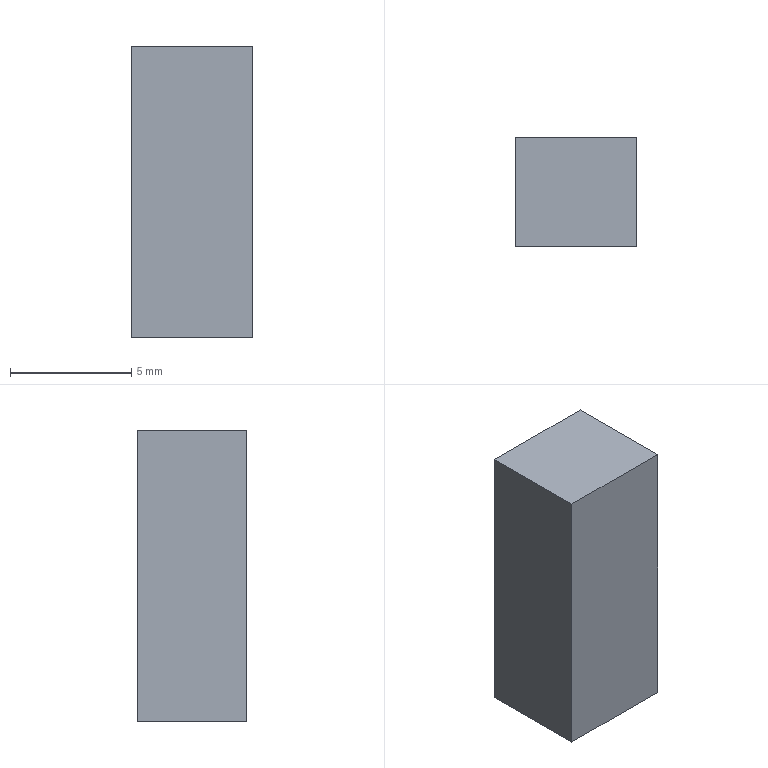Part | STEP file | Cuon T phu H01_7 | 1 solid | 6 faces | box 5 x 4.5 x 12 mm | volume 270 mm3 | plane 6
STEP:
#1=CARTESIAN_POINT('',(0.,0.,0.));
#2=DIRECTION('',(0.,0.,1.));
#3=DIRECTION('',(1.,0.,0.));
#4=AXIS2_PLACEMENT_3D('',#1,#2,#3);
#5=CARTESIAN_POINT('',(-2.5,2.25,-6.));
#6=VERTEX_POINT('',#5);
#7=CARTESIAN_POINT('',(-2.5,-2.25,-6.));
#8=VERTEX_POINT('',#7);
#9=CARTESIAN_POINT('',(-2.5,2.25,-6.));
#10=DIRECTION('',(0.,-1.,0.));
#11=VECTOR('',#10,1.);
#12=LINE('',#9,#11);
#13=CARTESIAN_POINT('',(-2.5,2.25,6.));
#14=DIRECTION('',(1.,0.,0.));
#15=DIRECTION('',(0.,1.,0.));
#16=AXIS2_PLACEMENT_3D('',#13,#14,#15);
#17=PLANE('',#16);
#18=CARTESIAN_POINT('',(0.,-12.));
#19=DIRECTION('',(-1.,0.));
#20=VECTOR('',#19,1.);
#21=LINE('',#18,#20);
#22=(GEOMETRIC_REPRESENTATION_CONTEXT(2)PARAMETRIC_REPRESENTATION_CONTEXT()REPRESENTATION_CONTEXT('',''));
#23=DEFINITIONAL_REPRESENTATION('',(#21),#22);
#24=PCURVE('',#17,#23);
#25=CARTESIAN_POINT('',(0.,0.,-6.));
#26=DIRECTION('',(0.,0.,1.));
#27=DIRECTION('',(1.,0.,0.));
#28=AXIS2_PLACEMENT_3D('',#25,#26,#27);
#29=PLANE('',#28);
#30=CARTESIAN_POINT('',(-2.5,2.25));
#31=DIRECTION('',(0.,-1.));
#32=VECTOR('',#31,1.);
#33=LINE('',#30,#32);
#34=(GEOMETRIC_REPRESENTATION_CONTEXT(2)PARAMETRIC_REPRESENTATION_CONTEXT()REPRESENTATION_CONTEXT('',''));
#35=DEFINITIONAL_REPRESENTATION('',(#33),#34);
#36=PCURVE('',#29,#35);
#37=SURFACE_CURVE('',#12,(#24,#36),.PCURVE_S1.);
#38=EDGE_CURVE('',#6,#8,#37,.T.);
#39=ORIENTED_EDGE('',*,*,#38,.T.);
#40=CARTESIAN_POINT('',(-2.5,-2.25,6.));
#41=VERTEX_POINT('',#40);
#42=CARTESIAN_POINT('',(-2.5,-2.25,6.));
#43=DIRECTION('',(0.,0.,-1.));
#44=VECTOR('',#43,1.);
#45=LINE('',#42,#44);
#46=CARTESIAN_POINT('',(-4.5,0.));
#47=DIRECTION('',(0.,-1.));
#48=VECTOR('',#47,1.);
#49=LINE('',#46,#48);
#50=(GEOMETRIC_REPRESENTATION_CONTEXT(2)PARAMETRIC_REPRESENTATION_CONTEXT()REPRESENTATION_CONTEXT('',''));
#51=DEFINITIONAL_REPRESENTATION('',(#49),#50);
#52=PCURVE('',#17,#51);
#53=CARTESIAN_POINT('',(-2.5,-2.25,6.));
#54=DIRECTION('',(0.,1.,0.));
#55=DIRECTION('',(0.,0.,1.));
#56=AXIS2_PLACEMENT_3D('',#53,#54,#55);
#57=PLANE('',#56);
#58=CARTESIAN_POINT('',(0.,0.));
#59=DIRECTION('',(-1.,0.));
#60=VECTOR('',#59,1.);
#61=LINE('',#58,#60);
#62=(GEOMETRIC_REPRESENTATION_CONTEXT(2)PARAMETRIC_REPRESENTATION_CONTEXT()REPRESENTATION_CONTEXT('',''));
#63=DEFINITIONAL_REPRESENTATION('',(#61),#62);
#64=PCURVE('',#57,#63);
#65=SURFACE_CURVE('',#45,(#52,#64),.PCURVE_S1.);
#66=EDGE_CURVE('',#41,#8,#65,.T.);
#67=ORIENTED_EDGE('',*,*,#66,.F.);
#68=CARTESIAN_POINT('',(-2.5,2.25,6.));
#69=VERTEX_POINT('',#68);
#70=CARTESIAN_POINT('',(-2.5,2.25,6.));
#71=DIRECTION('',(0.,-1.,0.));
#72=VECTOR('',#71,1.);
#73=LINE('',#70,#72);
#74=CARTESIAN_POINT('',(0.,0.));
#75=DIRECTION('',(-1.,0.));
#76=VECTOR('',#75,1.);
#77=LINE('',#74,#76);
#78=(GEOMETRIC_REPRESENTATION_CONTEXT(2)PARAMETRIC_REPRESENTATION_CONTEXT()REPRESENTATION_CONTEXT('',''));
#79=DEFINITIONAL_REPRESENTATION('',(#77),#78);
#80=PCURVE('',#17,#79);
#81=CARTESIAN_POINT('',(0.,0.,6.));
#82=DIRECTION('',(0.,0.,1.));
#83=DIRECTION('',(1.,0.,0.));
#84=AXIS2_PLACEMENT_3D('',#81,#82,#83);
#85=PLANE('',#84);
#86=CARTESIAN_POINT('',(-2.5,2.25));
#87=DIRECTION('',(0.,-1.));
#88=VECTOR('',#87,1.);
#89=LINE('',#86,#88);
#90=(GEOMETRIC_REPRESENTATION_CONTEXT(2)PARAMETRIC_REPRESENTATION_CONTEXT()REPRESENTATION_CONTEXT('',''));
#91=DEFINITIONAL_REPRESENTATION('',(#89),#90);
#92=PCURVE('',#85,#91);
#93=SURFACE_CURVE('',#73,(#80,#92),.PCURVE_S1.);
#94=EDGE_CURVE('',#69,#41,#93,.T.);
#95=ORIENTED_EDGE('',*,*,#94,.F.);
#96=CARTESIAN_POINT('',(-2.5,2.25,6.));
#97=DIRECTION('',(0.,0.,-1.));
#98=VECTOR('',#97,1.);
#99=LINE('',#96,#98);
#100=CARTESIAN_POINT('',(0.,0.));
#101=DIRECTION('',(0.,-1.));
#102=VECTOR('',#101,1.);
#103=LINE('',#100,#102);
#104=(GEOMETRIC_REPRESENTATION_CONTEXT(2)PARAMETRIC_REPRESENTATION_CONTEXT()REPRESENTATION_CONTEXT('',''));
#105=DEFINITIONAL_REPRESENTATION('',(#103),#104);
#106=PCURVE('',#17,#105);
#107=CARTESIAN_POINT('',(-2.5,2.25,6.));
#108=DIRECTION('',(0.,-1.,0.));
#109=DIRECTION('',(0.,0.,-1.));
#110=AXIS2_PLACEMENT_3D('',#107,#108,#109);
#111=PLANE('',#110);
#112=CARTESIAN_POINT('',(0.,0.));
#113=DIRECTION('',(1.,0.));
#114=VECTOR('',#113,1.);
#115=LINE('',#112,#114);
#116=(GEOMETRIC_REPRESENTATION_CONTEXT(2)PARAMETRIC_REPRESENTATION_CONTEXT()REPRESENTATION_CONTEXT('',''));
#117=DEFINITIONAL_REPRESENTATION('',(#115),#116);
#118=PCURVE('',#111,#117);
#119=SURFACE_CURVE('',#99,(#106,#118),.PCURVE_S1.);
#120=EDGE_CURVE('',#69,#6,#119,.T.);
#121=ORIENTED_EDGE('',*,*,#120,.T.);
#122=EDGE_LOOP('',(#39,#67,#95,#121));
#123=FACE_BOUND('',#122,.T.);
#124=ADVANCED_FACE('',(#123),#17,.F.);
#125=CARTESIAN_POINT('',(2.5,-2.25,-6.));
#126=VERTEX_POINT('',#125);
#127=CARTESIAN_POINT('',(-2.5,-2.25,-6.));
#128=DIRECTION('',(1.,0.,0.));
#129=VECTOR('',#128,1.);
#130=LINE('',#127,#129);
#131=CARTESIAN_POINT('',(-12.,0.));
#132=DIRECTION('',(0.,1.));
#133=VECTOR('',#132,1.);
#134=LINE('',#131,#133);
#135=(GEOMETRIC_REPRESENTATION_CONTEXT(2)PARAMETRIC_REPRESENTATION_CONTEXT()REPRESENTATION_CONTEXT('',''));
#136=DEFINITIONAL_REPRESENTATION('',(#134),#135);
#137=PCURVE('',#57,#136);
#138=CARTESIAN_POINT('',(-2.5,-2.25));
#139=DIRECTION('',(1.,0.));
#140=VECTOR('',#139,1.);
#141=LINE('',#138,#140);
#142=(GEOMETRIC_REPRESENTATION_CONTEXT(2)PARAMETRIC_REPRESENTATION_CONTEXT()REPRESENTATION_CONTEXT('',''));
#143=DEFINITIONAL_REPRESENTATION('',(#141),#142);
#144=PCURVE('',#29,#143);
#145=SURFACE_CURVE('',#130,(#137,#144),.PCURVE_S1.);
#146=EDGE_CURVE('',#8,#126,#145,.T.);
#147=ORIENTED_EDGE('',*,*,#146,.T.);
#148=CARTESIAN_POINT('',(2.5,-2.25,6.));
#149=VERTEX_POINT('',#148);
#150=CARTESIAN_POINT('',(2.5,-2.25,6.));
#151=DIRECTION('',(0.,0.,-1.));
#152=VECTOR('',#151,1.);
#153=LINE('',#150,#152);
#154=CARTESIAN_POINT('',(0.,5.));
#155=DIRECTION('',(-1.,0.));
#156=VECTOR('',#155,1.);
#157=LINE('',#154,#156);
#158=(GEOMETRIC_REPRESENTATION_CONTEXT(2)PARAMETRIC_REPRESENTATION_CONTEXT()REPRESENTATION_CONTEXT('',''));
#159=DEFINITIONAL_REPRESENTATION('',(#157),#158);
#160=PCURVE('',#57,#159);
#161=CARTESIAN_POINT('',(2.5,2.25,6.));
#162=DIRECTION('',(-1.,0.,0.));
#163=DIRECTION('',(0.,-1.,0.));
#164=AXIS2_PLACEMENT_3D('',#161,#162,#163);
#165=PLANE('',#164);
#166=CARTESIAN_POINT('',(4.5,0.));
#167=DIRECTION('',(0.,-1.));
#168=VECTOR('',#167,1.);
#169=LINE('',#166,#168);
#170=(GEOMETRIC_REPRESENTATION_CONTEXT(2)PARAMETRIC_REPRESENTATION_CONTEXT()REPRESENTATION_CONTEXT('',''));
#171=DEFINITIONAL_REPRESENTATION('',(#169),#170);
#172=PCURVE('',#165,#171);
#173=SURFACE_CURVE('',#153,(#160,#172),.PCURVE_S1.);
#174=EDGE_CURVE('',#149,#126,#173,.T.);
#175=ORIENTED_EDGE('',*,*,#174,.F.);
#176=CARTESIAN_POINT('',(-2.5,-2.25,6.));
#177=DIRECTION('',(1.,0.,0.));
#178=VECTOR('',#177,1.);
#179=LINE('',#176,#178);
#180=CARTESIAN_POINT('',(0.,0.));
#181=DIRECTION('',(0.,1.));
#182=VECTOR('',#181,1.);
#183=LINE('',#180,#182);
#184=(GEOMETRIC_REPRESENTATION_CONTEXT(2)PARAMETRIC_REPRESENTATION_CONTEXT()REPRESENTATION_CONTEXT('',''));
#185=DEFINITIONAL_REPRESENTATION('',(#183),#184);
#186=PCURVE('',#57,#185);
#187=CARTESIAN_POINT('',(-2.5,-2.25));
#188=DIRECTION('',(1.,0.));
#189=VECTOR('',#188,1.);
#190=LINE('',#187,#189);
#191=(GEOMETRIC_REPRESENTATION_CONTEXT(2)PARAMETRIC_REPRESENTATION_CONTEXT()REPRESENTATION_CONTEXT('',''));
#192=DEFINITIONAL_REPRESENTATION('',(#190),#191);
#193=PCURVE('',#85,#192);
#194=SURFACE_CURVE('',#179,(#186,#193),.PCURVE_S1.);
#195=EDGE_CURVE('',#41,#149,#194,.T.);
#196=ORIENTED_EDGE('',*,*,#195,.F.);
#197=ORIENTED_EDGE('',*,*,#66,.T.);
#198=EDGE_LOOP('',(#147,#175,#196,#197));
#199=FACE_BOUND('',#198,.T.);
#200=ADVANCED_FACE('',(#199),#57,.F.);
#201=CARTESIAN_POINT('',(2.5,2.25,-6.));
#202=VERTEX_POINT('',#201);
#203=CARTESIAN_POINT('',(2.5,2.25,-6.));
#204=DIRECTION('',(0.,1.,0.));
#205=VECTOR('',#204,1.);
#206=LINE('',#203,#205);
#207=CARTESIAN_POINT('',(0.,-12.));
#208=DIRECTION('',(-1.,0.));
#209=VECTOR('',#208,1.);
#210=LINE('',#207,#209);
#211=(GEOMETRIC_REPRESENTATION_CONTEXT(2)PARAMETRIC_REPRESENTATION_CONTEXT()REPRESENTATION_CONTEXT('',''));
#212=DEFINITIONAL_REPRESENTATION('',(#210),#211);
#213=PCURVE('',#165,#212);
#214=CARTESIAN_POINT('',(2.5,2.25));
#215=DIRECTION('',(0.,1.));
#216=VECTOR('',#215,1.);
#217=LINE('',#214,#216);
#218=(GEOMETRIC_REPRESENTATION_CONTEXT(2)PARAMETRIC_REPRESENTATION_CONTEXT()REPRESENTATION_CONTEXT('',''));
#219=DEFINITIONAL_REPRESENTATION('',(#217),#218);
#220=PCURVE('',#29,#219);
#221=SURFACE_CURVE('',#206,(#213,#220),.PCURVE_S1.);
#222=EDGE_CURVE('',#126,#202,#221,.T.);
#223=ORIENTED_EDGE('',*,*,#222,.T.);
#224=CARTESIAN_POINT('',(2.5,2.25,6.));
#225=VERTEX_POINT('',#224);
#226=CARTESIAN_POINT('',(2.5,2.25,6.));
#227=DIRECTION('',(0.,0.,-1.));
#228=VECTOR('',#227,1.);
#229=LINE('',#226,#228);
#230=CARTESIAN_POINT('',(0.,0.));
#231=DIRECTION('',(0.,-1.));
#232=VECTOR('',#231,1.);
#233=LINE('',#230,#232);
#234=(GEOMETRIC_REPRESENTATION_CONTEXT(2)PARAMETRIC_REPRESENTATION_CONTEXT()REPRESENTATION_CONTEXT('',''));
#235=DEFINITIONAL_REPRESENTATION('',(#233),#234);
#236=PCURVE('',#165,#235);
#237=CARTESIAN_POINT('',(0.,5.));
#238=DIRECTION('',(1.,0.));
#239=VECTOR('',#238,1.);
#240=LINE('',#237,#239);
#241=(GEOMETRIC_REPRESENTATION_CONTEXT(2)PARAMETRIC_REPRESENTATION_CONTEXT()REPRESENTATION_CONTEXT('',''));
#242=DEFINITIONAL_REPRESENTATION('',(#240),#241);
#243=PCURVE('',#111,#242);
#244=SURFACE_CURVE('',#229,(#236,#243),.PCURVE_S1.);
#245=EDGE_CURVE('',#225,#202,#244,.T.);
#246=ORIENTED_EDGE('',*,*,#245,.F.);
#247=CARTESIAN_POINT('',(2.5,2.25,6.));
#248=DIRECTION('',(0.,1.,0.));
#249=VECTOR('',#248,1.);
#250=LINE('',#247,#249);
#251=CARTESIAN_POINT('',(0.,0.));
#252=DIRECTION('',(-1.,0.));
#253=VECTOR('',#252,1.);
#254=LINE('',#251,#253);
#255=(GEOMETRIC_REPRESENTATION_CONTEXT(2)PARAMETRIC_REPRESENTATION_CONTEXT()REPRESENTATION_CONTEXT('',''));
#256=DEFINITIONAL_REPRESENTATION('',(#254),#255);
#257=PCURVE('',#165,#256);
#258=CARTESIAN_POINT('',(2.5,2.25));
#259=DIRECTION('',(0.,1.));
#260=VECTOR('',#259,1.);
#261=LINE('',#258,#260);
#262=(GEOMETRIC_REPRESENTATION_CONTEXT(2)PARAMETRIC_REPRESENTATION_CONTEXT()REPRESENTATION_CONTEXT('',''));
#263=DEFINITIONAL_REPRESENTATION('',(#261),#262);
#264=PCURVE('',#85,#263);
#265=SURFACE_CURVE('',#250,(#257,#264),.PCURVE_S1.);
#266=EDGE_CURVE('',#149,#225,#265,.T.);
#267=ORIENTED_EDGE('',*,*,#266,.F.);
#268=ORIENTED_EDGE('',*,*,#174,.T.);
#269=EDGE_LOOP('',(#223,#246,#267,#268));
#270=FACE_BOUND('',#269,.T.);
#271=ADVANCED_FACE('',(#270),#165,.F.);
#272=CARTESIAN_POINT('',(-2.5,2.25,-6.));
#273=DIRECTION('',(-1.,0.,0.));
#274=VECTOR('',#273,1.);
#275=LINE('',#272,#274);
#276=CARTESIAN_POINT('',(12.,0.));
#277=DIRECTION('',(0.,-1.));
#278=VECTOR('',#277,1.);
#279=LINE('',#276,#278);
#280=(GEOMETRIC_REPRESENTATION_CONTEXT(2)PARAMETRIC_REPRESENTATION_CONTEXT()REPRESENTATION_CONTEXT('',''));
#281=DEFINITIONAL_REPRESENTATION('',(#279),#280);
#282=PCURVE('',#111,#281);
#283=CARTESIAN_POINT('',(-2.5,2.25));
#284=DIRECTION('',(-1.,0.));
#285=VECTOR('',#284,1.);
#286=LINE('',#283,#285);
#287=(GEOMETRIC_REPRESENTATION_CONTEXT(2)PARAMETRIC_REPRESENTATION_CONTEXT()REPRESENTATION_CONTEXT('',''));
#288=DEFINITIONAL_REPRESENTATION('',(#286),#287);
#289=PCURVE('',#29,#288);
#290=SURFACE_CURVE('',#275,(#282,#289),.PCURVE_S1.);
#291=EDGE_CURVE('',#202,#6,#290,.T.);
#292=ORIENTED_EDGE('',*,*,#291,.T.);
#293=ORIENTED_EDGE('',*,*,#120,.F.);
#294=CARTESIAN_POINT('',(-2.5,2.25,6.));
#295=DIRECTION('',(-1.,0.,0.));
#296=VECTOR('',#295,1.);
#297=LINE('',#294,#296);
#298=CARTESIAN_POINT('',(0.,0.));
#299=DIRECTION('',(0.,-1.));
#300=VECTOR('',#299,1.);
#301=LINE('',#298,#300);
#302=(GEOMETRIC_REPRESENTATION_CONTEXT(2)PARAMETRIC_REPRESENTATION_CONTEXT()REPRESENTATION_CONTEXT('',''));
#303=DEFINITIONAL_REPRESENTATION('',(#301),#302);
#304=PCURVE('',#111,#303);
#305=CARTESIAN_POINT('',(-2.5,2.25));
#306=DIRECTION('',(-1.,0.));
#307=VECTOR('',#306,1.);
#308=LINE('',#305,#307);
#309=(GEOMETRIC_REPRESENTATION_CONTEXT(2)PARAMETRIC_REPRESENTATION_CONTEXT()REPRESENTATION_CONTEXT('',''));
#310=DEFINITIONAL_REPRESENTATION('',(#308),#309);
#311=PCURVE('',#85,#310);
#312=SURFACE_CURVE('',#297,(#304,#311),.PCURVE_S1.);
#313=EDGE_CURVE('',#225,#69,#312,.T.);
#314=ORIENTED_EDGE('',*,*,#313,.F.);
#315=ORIENTED_EDGE('',*,*,#245,.T.);
#316=EDGE_LOOP('',(#292,#293,#314,#315));
#317=FACE_BOUND('',#316,.T.);
#318=ADVANCED_FACE('',(#317),#111,.F.);
#319=ORIENTED_EDGE('',*,*,#94,.T.);
#320=ORIENTED_EDGE('',*,*,#195,.T.);
#321=ORIENTED_EDGE('',*,*,#266,.T.);
#322=ORIENTED_EDGE('',*,*,#313,.T.);
#323=EDGE_LOOP('',(#319,#320,#321,#322));
#324=FACE_BOUND('',#323,.T.);
#325=ADVANCED_FACE('',(#324),#85,.T.);
#326=ORIENTED_EDGE('',*,*,#38,.F.);
#327=ORIENTED_EDGE('',*,*,#291,.F.);
#328=ORIENTED_EDGE('',*,*,#222,.F.);
#329=ORIENTED_EDGE('',*,*,#146,.F.);
#330=EDGE_LOOP('',(#326,#327,#328,#329));
#331=FACE_BOUND('',#330,.T.);
#332=ADVANCED_FACE('',(#331),#29,.F.);
#333=CLOSED_SHELL('',(#124,#200,#271,#318,#325,#332));
#334=MANIFOLD_SOLID_BREP('',#333);
#335=(LENGTH_UNIT()NAMED_UNIT(*)SI_UNIT(.MILLI.,.METRE.));
#336=UNCERTAINTY_MEASURE_WITH_UNIT(LENGTH_MEASURE(0.0000001),#335,'','');
#337=(NAMED_UNIT(*)PLANE_ANGLE_UNIT()SI_UNIT($,.RADIAN.));
#338=(NAMED_UNIT(*)SI_UNIT($,.STERADIAN.)SOLID_ANGLE_UNIT());
#339=(GEOMETRIC_REPRESENTATION_CONTEXT(3)GLOBAL_UNCERTAINTY_ASSIGNED_CONTEXT((#336))GLOBAL_UNIT_ASSIGNED_CONTEXT((#335,#337,#338))REPRESENTATION_CONTEXT('',''));
#340=ADVANCED_BREP_SHAPE_REPRESENTATION('',(#4,#334),#339);